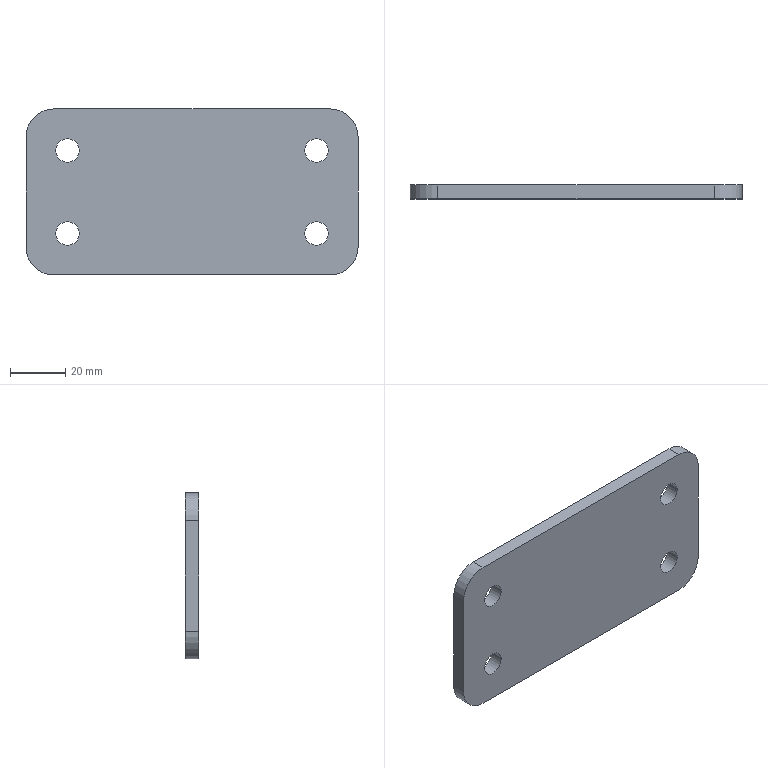Part | STEP file | JBJ-P-1007-05 | 1 solid | 14 faces | box 120 x 5 x 60 mm | volume 34436 mm3 | cylinder 8 | plane 6 | commonest cylinder face diameters 8.5 x4 20 x4
STEP:
#1=CARTESIAN_POINT('',(105.,5.,49.25));
#2=VERTEX_POINT('',#1);
#3=CARTESIAN_POINT('',(105.,5.,45.));
#4=DIRECTION('',(0.,1.,0.));
#5=DIRECTION('',(0.,0.,1.));
#6=AXIS2_PLACEMENT_3D('',#3,#4,#5);
#7=CIRCLE('',#6,4.25);
#8=EDGE_CURVE('',#2,#2,#7,.T.);
#9=ORIENTED_EDGE('',*,*,#8,.F.);
#10=EDGE_LOOP('',(#9));
#11=FACE_BOUND('',#10,.T.);
#12=CARTESIAN_POINT('',(15.,5.,19.25));
#13=VERTEX_POINT('',#12);
#14=CARTESIAN_POINT('',(15.,5.,15.));
#15=DIRECTION('',(0.,1.,0.));
#16=DIRECTION('',(0.,0.,1.));
#17=AXIS2_PLACEMENT_3D('',#14,#15,#16);
#18=CIRCLE('',#17,4.25);
#19=EDGE_CURVE('',#13,#13,#18,.T.);
#20=ORIENTED_EDGE('',*,*,#19,.F.);
#21=EDGE_LOOP('',(#20));
#22=FACE_BOUND('',#21,.T.);
#23=CARTESIAN_POINT('',(0.,5.,10.));
#24=VERTEX_POINT('',#23);
#25=CARTESIAN_POINT('',(0.,5.,50.));
#26=VERTEX_POINT('',#25);
#27=CARTESIAN_POINT('',(0.,5.,0.));
#28=DIRECTION('',(0.,0.,1.));
#29=VECTOR('',#28,1000.);
#30=LINE('',#27,#29);
#31=EDGE_CURVE('',#24,#26,#30,.T.);
#32=ORIENTED_EDGE('',*,*,#31,.T.);
#33=CARTESIAN_POINT('',(10.,5.,60.));
#34=VERTEX_POINT('',#33);
#35=CARTESIAN_POINT('',(10.,5.,50.));
#36=DIRECTION('',(0.,1.,0.));
#37=DIRECTION('',(0.,0.,1.));
#38=AXIS2_PLACEMENT_3D('',#35,#36,#37);
#39=CIRCLE('',#38,10.);
#40=EDGE_CURVE('',#26,#34,#39,.T.);
#41=ORIENTED_EDGE('',*,*,#40,.T.);
#42=CARTESIAN_POINT('',(110.,5.,60.));
#43=VERTEX_POINT('',#42);
#44=CARTESIAN_POINT('',(0.,5.,60.));
#45=DIRECTION('',(1.,0.,0.));
#46=VECTOR('',#45,1000.);
#47=LINE('',#44,#46);
#48=EDGE_CURVE('',#34,#43,#47,.T.);
#49=ORIENTED_EDGE('',*,*,#48,.T.);
#50=CARTESIAN_POINT('',(120.,5.,50.));
#51=VERTEX_POINT('',#50);
#52=CARTESIAN_POINT('',(110.,5.,50.));
#53=DIRECTION('',(0.,1.,0.));
#54=DIRECTION('',(0.,0.,1.));
#55=AXIS2_PLACEMENT_3D('',#52,#53,#54);
#56=CIRCLE('',#55,10.);
#57=EDGE_CURVE('',#43,#51,#56,.T.);
#58=ORIENTED_EDGE('',*,*,#57,.T.);
#59=CARTESIAN_POINT('',(120.,5.,10.));
#60=VERTEX_POINT('',#59);
#61=CARTESIAN_POINT('',(120.,5.,0.));
#62=DIRECTION('',(0.,0.,-1.));
#63=VECTOR('',#62,1000.);
#64=LINE('',#61,#63);
#65=EDGE_CURVE('',#51,#60,#64,.T.);
#66=ORIENTED_EDGE('',*,*,#65,.T.);
#67=CARTESIAN_POINT('',(110.,5.,0.));
#68=VERTEX_POINT('',#67);
#69=CARTESIAN_POINT('',(110.,5.,10.));
#70=DIRECTION('',(0.,1.,0.));
#71=DIRECTION('',(0.,0.,1.));
#72=AXIS2_PLACEMENT_3D('',#69,#70,#71);
#73=CIRCLE('',#72,10.);
#74=EDGE_CURVE('',#60,#68,#73,.T.);
#75=ORIENTED_EDGE('',*,*,#74,.T.);
#76=CARTESIAN_POINT('',(10.,5.,0.));
#77=VERTEX_POINT('',#76);
#78=CARTESIAN_POINT('',(0.,5.,0.));
#79=DIRECTION('',(-1.,0.,0.));
#80=VECTOR('',#79,1000.);
#81=LINE('',#78,#80);
#82=EDGE_CURVE('',#68,#77,#81,.T.);
#83=ORIENTED_EDGE('',*,*,#82,.T.);
#84=CARTESIAN_POINT('',(10.,5.,10.));
#85=DIRECTION('',(0.,1.,0.));
#86=DIRECTION('',(0.,0.,1.));
#87=AXIS2_PLACEMENT_3D('',#84,#85,#86);
#88=CIRCLE('',#87,10.);
#89=EDGE_CURVE('',#77,#24,#88,.T.);
#90=ORIENTED_EDGE('',*,*,#89,.T.);
#91=EDGE_LOOP('',(#32,#41,#49,#58,#66,#75,#83,#90));
#92=FACE_OUTER_BOUND('',#91,.T.);
#93=CARTESIAN_POINT('',(15.,5.,40.75));
#94=VERTEX_POINT('',#93);
#95=CARTESIAN_POINT('',(15.,5.,45.));
#96=DIRECTION('',(0.,1.,0.));
#97=DIRECTION('',(0.,0.,-1.));
#98=AXIS2_PLACEMENT_3D('',#95,#96,#97);
#99=CIRCLE('',#98,4.25);
#100=EDGE_CURVE('',#94,#94,#99,.T.);
#101=ORIENTED_EDGE('',*,*,#100,.F.);
#102=EDGE_LOOP('',(#101));
#103=FACE_BOUND('',#102,.T.);
#104=CARTESIAN_POINT('',(105.,5.,10.75));
#105=VERTEX_POINT('',#104);
#106=CARTESIAN_POINT('',(105.,5.,15.));
#107=DIRECTION('',(0.,1.,0.));
#108=DIRECTION('',(0.,0.,-1.));
#109=AXIS2_PLACEMENT_3D('',#106,#107,#108);
#110=CIRCLE('',#109,4.25);
#111=EDGE_CURVE('',#105,#105,#110,.T.);
#112=ORIENTED_EDGE('',*,*,#111,.F.);
#113=EDGE_LOOP('',(#112));
#114=FACE_BOUND('',#113,.T.);
#115=CARTESIAN_POINT('',(0.,5.,0.));
#116=DIRECTION('',(0.,1.,0.));
#117=DIRECTION('',(0.,0.,1.));
#118=AXIS2_PLACEMENT_3D('',#115,#116,#117);
#119=PLANE('',#118);
#120=ADVANCED_FACE('',(#11,#22,#92,#103,#114),#119,.T.);
#121=CARTESIAN_POINT('',(10.,0.,60.));
#122=VERTEX_POINT('',#121);
#123=CARTESIAN_POINT('',(110.,0.,60.));
#124=VERTEX_POINT('',#123);
#125=CARTESIAN_POINT('',(0.,0.,60.));
#126=DIRECTION('',(1.,0.,0.));
#127=VECTOR('',#126,1000.);
#128=LINE('',#125,#127);
#129=EDGE_CURVE('',#122,#124,#128,.T.);
#130=ORIENTED_EDGE('',*,*,#129,.F.);
#131=CARTESIAN_POINT('',(0.,0.,50.));
#132=VERTEX_POINT('',#131);
#133=CARTESIAN_POINT('',(10.,0.,50.));
#134=DIRECTION('',(0.,-1.,0.));
#135=DIRECTION('',(0.,0.,1.));
#136=AXIS2_PLACEMENT_3D('',#133,#134,#135);
#137=CIRCLE('',#136,10.);
#138=EDGE_CURVE('',#122,#132,#137,.T.);
#139=ORIENTED_EDGE('',*,*,#138,.T.);
#140=CARTESIAN_POINT('',(0.,0.,10.));
#141=VERTEX_POINT('',#140);
#142=CARTESIAN_POINT('',(0.,0.,0.));
#143=DIRECTION('',(0.,0.,1.));
#144=VECTOR('',#143,1000.);
#145=LINE('',#142,#144);
#146=EDGE_CURVE('',#141,#132,#145,.T.);
#147=ORIENTED_EDGE('',*,*,#146,.F.);
#148=CARTESIAN_POINT('',(10.,0.,0.));
#149=VERTEX_POINT('',#148);
#150=CARTESIAN_POINT('',(10.,0.,10.));
#151=DIRECTION('',(0.,-1.,0.));
#152=DIRECTION('',(0.,0.,1.));
#153=AXIS2_PLACEMENT_3D('',#150,#151,#152);
#154=CIRCLE('',#153,10.);
#155=EDGE_CURVE('',#141,#149,#154,.T.);
#156=ORIENTED_EDGE('',*,*,#155,.T.);
#157=CARTESIAN_POINT('',(110.,0.,0.));
#158=VERTEX_POINT('',#157);
#159=CARTESIAN_POINT('',(0.,0.,0.));
#160=DIRECTION('',(-1.,0.,0.));
#161=VECTOR('',#160,1000.);
#162=LINE('',#159,#161);
#163=EDGE_CURVE('',#158,#149,#162,.T.);
#164=ORIENTED_EDGE('',*,*,#163,.F.);
#165=CARTESIAN_POINT('',(120.,0.,10.));
#166=VERTEX_POINT('',#165);
#167=CARTESIAN_POINT('',(110.,0.,10.));
#168=DIRECTION('',(0.,-1.,0.));
#169=DIRECTION('',(0.,0.,1.));
#170=AXIS2_PLACEMENT_3D('',#167,#168,#169);
#171=CIRCLE('',#170,10.);
#172=EDGE_CURVE('',#158,#166,#171,.T.);
#173=ORIENTED_EDGE('',*,*,#172,.T.);
#174=CARTESIAN_POINT('',(120.,0.,50.));
#175=VERTEX_POINT('',#174);
#176=CARTESIAN_POINT('',(120.,0.,0.));
#177=DIRECTION('',(0.,0.,-1.));
#178=VECTOR('',#177,1000.);
#179=LINE('',#176,#178);
#180=EDGE_CURVE('',#175,#166,#179,.T.);
#181=ORIENTED_EDGE('',*,*,#180,.F.);
#182=CARTESIAN_POINT('',(110.,0.,50.));
#183=DIRECTION('',(0.,-1.,0.));
#184=DIRECTION('',(0.,0.,1.));
#185=AXIS2_PLACEMENT_3D('',#182,#183,#184);
#186=CIRCLE('',#185,10.);
#187=EDGE_CURVE('',#175,#124,#186,.T.);
#188=ORIENTED_EDGE('',*,*,#187,.T.);
#189=EDGE_LOOP('',(#130,#139,#147,#156,#164,#173,#181,#188));
#190=FACE_OUTER_BOUND('',#189,.T.);
#191=CARTESIAN_POINT('',(15.,0.,19.25));
#192=VERTEX_POINT('',#191);
#193=CARTESIAN_POINT('',(15.,0.,15.));
#194=DIRECTION('',(0.,1.,0.));
#195=DIRECTION('',(0.,0.,1.));
#196=AXIS2_PLACEMENT_3D('',#193,#194,#195);
#197=CIRCLE('',#196,4.25);
#198=EDGE_CURVE('',#192,#192,#197,.T.);
#199=ORIENTED_EDGE('',*,*,#198,.T.);
#200=EDGE_LOOP('',(#199));
#201=FACE_BOUND('',#200,.T.);
#202=CARTESIAN_POINT('',(15.,0.,40.75));
#203=VERTEX_POINT('',#202);
#204=CARTESIAN_POINT('',(15.,0.,45.));
#205=DIRECTION('',(0.,1.,0.));
#206=DIRECTION('',(0.,0.,-1.));
#207=AXIS2_PLACEMENT_3D('',#204,#205,#206);
#208=CIRCLE('',#207,4.25);
#209=EDGE_CURVE('',#203,#203,#208,.T.);
#210=ORIENTED_EDGE('',*,*,#209,.T.);
#211=EDGE_LOOP('',(#210));
#212=FACE_BOUND('',#211,.T.);
#213=CARTESIAN_POINT('',(105.,0.,49.25));
#214=VERTEX_POINT('',#213);
#215=CARTESIAN_POINT('',(105.,0.,45.));
#216=DIRECTION('',(0.,1.,0.));
#217=DIRECTION('',(0.,0.,1.));
#218=AXIS2_PLACEMENT_3D('',#215,#216,#217);
#219=CIRCLE('',#218,4.25);
#220=EDGE_CURVE('',#214,#214,#219,.T.);
#221=ORIENTED_EDGE('',*,*,#220,.T.);
#222=EDGE_LOOP('',(#221));
#223=FACE_BOUND('',#222,.T.);
#224=CARTESIAN_POINT('',(105.,0.,10.75));
#225=VERTEX_POINT('',#224);
#226=CARTESIAN_POINT('',(105.,0.,15.));
#227=DIRECTION('',(0.,1.,0.));
#228=DIRECTION('',(0.,0.,-1.));
#229=AXIS2_PLACEMENT_3D('',#226,#227,#228);
#230=CIRCLE('',#229,4.25);
#231=EDGE_CURVE('',#225,#225,#230,.T.);
#232=ORIENTED_EDGE('',*,*,#231,.T.);
#233=EDGE_LOOP('',(#232));
#234=FACE_BOUND('',#233,.T.);
#235=CARTESIAN_POINT('',(0.,0.,0.));
#236=DIRECTION('',(0.,1.,0.));
#237=DIRECTION('',(0.,0.,1.));
#238=AXIS2_PLACEMENT_3D('',#235,#236,#237);
#239=PLANE('',#238);
#240=ADVANCED_FACE('',(#190,#201,#212,#223,#234),#239,.F.);
#241=ORIENTED_EDGE('',*,*,#146,.T.);
#242=CARTESIAN_POINT('',(0.,5.,50.));
#243=DIRECTION('',(0.,1.,0.));
#244=VECTOR('',#243,1000.);
#245=LINE('',#242,#244);
#246=EDGE_CURVE('',#132,#26,#245,.T.);
#247=ORIENTED_EDGE('',*,*,#246,.T.);
#248=ORIENTED_EDGE('',*,*,#31,.F.);
#249=CARTESIAN_POINT('',(0.,5.,10.));
#250=DIRECTION('',(0.,-1.,0.));
#251=VECTOR('',#250,1000.);
#252=LINE('',#249,#251);
#253=EDGE_CURVE('',#24,#141,#252,.T.);
#254=ORIENTED_EDGE('',*,*,#253,.T.);
#255=EDGE_LOOP('',(#241,#247,#248,#254));
#256=FACE_OUTER_BOUND('',#255,.T.);
#257=CARTESIAN_POINT('',(0.,5.,0.));
#258=DIRECTION('',(1.,0.,0.));
#259=DIRECTION('',(0.,0.,-1.));
#260=AXIS2_PLACEMENT_3D('',#257,#258,#259);
#261=PLANE('',#260);
#262=ADVANCED_FACE('',(#256),#261,.F.);
#263=ORIENTED_EDGE('',*,*,#48,.F.);
#264=CARTESIAN_POINT('',(10.,5.,60.));
#265=DIRECTION('',(0.,-1.,0.));
#266=VECTOR('',#265,1000.);
#267=LINE('',#264,#266);
#268=EDGE_CURVE('',#34,#122,#267,.T.);
#269=ORIENTED_EDGE('',*,*,#268,.T.);
#270=ORIENTED_EDGE('',*,*,#129,.T.);
#271=CARTESIAN_POINT('',(110.,5.,60.));
#272=DIRECTION('',(0.,1.,0.));
#273=VECTOR('',#272,1000.);
#274=LINE('',#271,#273);
#275=EDGE_CURVE('',#124,#43,#274,.T.);
#276=ORIENTED_EDGE('',*,*,#275,.T.);
#277=EDGE_LOOP('',(#263,#269,#270,#276));
#278=FACE_OUTER_BOUND('',#277,.T.);
#279=CARTESIAN_POINT('',(0.,5.,60.));
#280=DIRECTION('',(0.,0.,-1.));
#281=DIRECTION('',(-1.,0.,0.));
#282=AXIS2_PLACEMENT_3D('',#279,#280,#281);
#283=PLANE('',#282);
#284=ADVANCED_FACE('',(#278),#283,.F.);
#285=ORIENTED_EDGE('',*,*,#180,.T.);
#286=CARTESIAN_POINT('',(120.,5.,10.));
#287=DIRECTION('',(0.,1.,0.));
#288=VECTOR('',#287,1000.);
#289=LINE('',#286,#288);
#290=EDGE_CURVE('',#166,#60,#289,.T.);
#291=ORIENTED_EDGE('',*,*,#290,.T.);
#292=ORIENTED_EDGE('',*,*,#65,.F.);
#293=CARTESIAN_POINT('',(120.,5.,50.));
#294=DIRECTION('',(0.,-1.,0.));
#295=VECTOR('',#294,1000.);
#296=LINE('',#293,#295);
#297=EDGE_CURVE('',#51,#175,#296,.T.);
#298=ORIENTED_EDGE('',*,*,#297,.T.);
#299=EDGE_LOOP('',(#285,#291,#292,#298));
#300=FACE_OUTER_BOUND('',#299,.T.);
#301=CARTESIAN_POINT('',(120.,5.,0.));
#302=DIRECTION('',(-1.,0.,0.));
#303=DIRECTION('',(0.,0.,1.));
#304=AXIS2_PLACEMENT_3D('',#301,#302,#303);
#305=PLANE('',#304);
#306=ADVANCED_FACE('',(#300),#305,.F.);
#307=ORIENTED_EDGE('',*,*,#163,.T.);
#308=CARTESIAN_POINT('',(10.,5.,0.));
#309=DIRECTION('',(0.,1.,0.));
#310=VECTOR('',#309,1000.);
#311=LINE('',#308,#310);
#312=EDGE_CURVE('',#149,#77,#311,.T.);
#313=ORIENTED_EDGE('',*,*,#312,.T.);
#314=ORIENTED_EDGE('',*,*,#82,.F.);
#315=CARTESIAN_POINT('',(110.,5.,0.));
#316=DIRECTION('',(0.,-1.,0.));
#317=VECTOR('',#316,1000.);
#318=LINE('',#315,#317);
#319=EDGE_CURVE('',#68,#158,#318,.T.);
#320=ORIENTED_EDGE('',*,*,#319,.T.);
#321=EDGE_LOOP('',(#307,#313,#314,#320));
#322=FACE_OUTER_BOUND('',#321,.T.);
#323=CARTESIAN_POINT('',(0.,5.,0.));
#324=DIRECTION('',(0.,0.,1.));
#325=DIRECTION('',(1.,0.,0.));
#326=AXIS2_PLACEMENT_3D('',#323,#324,#325);
#327=PLANE('',#326);
#328=ADVANCED_FACE('',(#322),#327,.F.);
#329=ORIENTED_EDGE('',*,*,#19,.T.);
#330=EDGE_LOOP('',(#329));
#331=FACE_OUTER_BOUND('',#330,.T.);
#332=ORIENTED_EDGE('',*,*,#198,.F.);
#333=EDGE_LOOP('',(#332));
#334=FACE_OUTER_BOUND('',#333,.T.);
#335=CARTESIAN_POINT('',(15.,5.,15.));
#336=DIRECTION('',(0.,-1.,0.));
#337=DIRECTION('',(0.,0.,-1.));
#338=AXIS2_PLACEMENT_3D('',#335,#336,#337);
#339=CYLINDRICAL_SURFACE('',#338,4.25);
#340=ADVANCED_FACE('',(#331,#334),#339,.F.);
#341=ORIENTED_EDGE('',*,*,#100,.T.);
#342=EDGE_LOOP('',(#341));
#343=FACE_OUTER_BOUND('',#342,.T.);
#344=ORIENTED_EDGE('',*,*,#209,.F.);
#345=EDGE_LOOP('',(#344));
#346=FACE_OUTER_BOUND('',#345,.T.);
#347=CARTESIAN_POINT('',(15.,5.,45.));
#348=DIRECTION('',(0.,-1.,0.));
#349=DIRECTION('',(0.,0.,-1.));
#350=AXIS2_PLACEMENT_3D('',#347,#348,#349);
#351=CYLINDRICAL_SURFACE('',#350,4.25);
#352=ADVANCED_FACE('',(#343,#346),#351,.F.);
#353=ORIENTED_EDGE('',*,*,#8,.T.);
#354=EDGE_LOOP('',(#353));
#355=FACE_OUTER_BOUND('',#354,.T.);
#356=ORIENTED_EDGE('',*,*,#220,.F.);
#357=EDGE_LOOP('',(#356));
#358=FACE_OUTER_BOUND('',#357,.T.);
#359=CARTESIAN_POINT('',(105.,5.,45.));
#360=DIRECTION('',(0.,-1.,0.));
#361=DIRECTION('',(0.,0.,-1.));
#362=AXIS2_PLACEMENT_3D('',#359,#360,#361);
#363=CYLINDRICAL_SURFACE('',#362,4.25);
#364=ADVANCED_FACE('',(#355,#358),#363,.F.);
#365=ORIENTED_EDGE('',*,*,#111,.T.);
#366=EDGE_LOOP('',(#365));
#367=FACE_OUTER_BOUND('',#366,.T.);
#368=ORIENTED_EDGE('',*,*,#231,.F.);
#369=EDGE_LOOP('',(#368));
#370=FACE_OUTER_BOUND('',#369,.T.);
#371=CARTESIAN_POINT('',(105.,5.,15.));
#372=DIRECTION('',(0.,-1.,0.));
#373=DIRECTION('',(0.,0.,-1.));
#374=AXIS2_PLACEMENT_3D('',#371,#372,#373);
#375=CYLINDRICAL_SURFACE('',#374,4.25);
#376=ADVANCED_FACE('',(#367,#370),#375,.F.);
#377=ORIENTED_EDGE('',*,*,#40,.F.);
#378=ORIENTED_EDGE('',*,*,#246,.F.);
#379=ORIENTED_EDGE('',*,*,#138,.F.);
#380=ORIENTED_EDGE('',*,*,#268,.F.);
#381=EDGE_LOOP('',(#377,#378,#379,#380));
#382=FACE_OUTER_BOUND('',#381,.T.);
#383=CARTESIAN_POINT('',(10.,5.,50.));
#384=DIRECTION('',(0.,-1.,0.));
#385=DIRECTION('',(0.,0.,-1.));
#386=AXIS2_PLACEMENT_3D('',#383,#384,#385);
#387=CYLINDRICAL_SURFACE('',#386,10.);
#388=ADVANCED_FACE('',(#382),#387,.T.);
#389=ORIENTED_EDGE('',*,*,#89,.F.);
#390=ORIENTED_EDGE('',*,*,#312,.F.);
#391=ORIENTED_EDGE('',*,*,#155,.F.);
#392=ORIENTED_EDGE('',*,*,#253,.F.);
#393=EDGE_LOOP('',(#389,#390,#391,#392));
#394=FACE_OUTER_BOUND('',#393,.T.);
#395=CARTESIAN_POINT('',(10.,5.,10.));
#396=DIRECTION('',(0.,-1.,0.));
#397=DIRECTION('',(0.,0.,-1.));
#398=AXIS2_PLACEMENT_3D('',#395,#396,#397);
#399=CYLINDRICAL_SURFACE('',#398,10.);
#400=ADVANCED_FACE('',(#394),#399,.T.);
#401=ORIENTED_EDGE('',*,*,#74,.F.);
#402=ORIENTED_EDGE('',*,*,#290,.F.);
#403=ORIENTED_EDGE('',*,*,#172,.F.);
#404=ORIENTED_EDGE('',*,*,#319,.F.);
#405=EDGE_LOOP('',(#401,#402,#403,#404));
#406=FACE_OUTER_BOUND('',#405,.T.);
#407=CARTESIAN_POINT('',(110.,5.,10.));
#408=DIRECTION('',(0.,-1.,0.));
#409=DIRECTION('',(0.,0.,-1.));
#410=AXIS2_PLACEMENT_3D('',#407,#408,#409);
#411=CYLINDRICAL_SURFACE('',#410,10.);
#412=ADVANCED_FACE('',(#406),#411,.T.);
#413=ORIENTED_EDGE('',*,*,#57,.F.);
#414=ORIENTED_EDGE('',*,*,#275,.F.);
#415=ORIENTED_EDGE('',*,*,#187,.F.);
#416=ORIENTED_EDGE('',*,*,#297,.F.);
#417=EDGE_LOOP('',(#413,#414,#415,#416));
#418=FACE_OUTER_BOUND('',#417,.T.);
#419=CARTESIAN_POINT('',(110.,5.,50.));
#420=DIRECTION('',(0.,-1.,0.));
#421=DIRECTION('',(0.,0.,-1.));
#422=AXIS2_PLACEMENT_3D('',#419,#420,#421);
#423=CYLINDRICAL_SURFACE('',#422,10.);
#424=ADVANCED_FACE('',(#418),#423,.T.);
#425=CLOSED_SHELL('',(#120,#240,#262,#284,#306,#328,#340,#352,#364,#376,#388,#400,#412,#424));
#426=MANIFOLD_SOLID_BREP('',#425);
#427=CARTESIAN_POINT('',(0.,0.,0.));
#428=DIRECTION('',(0.,0.,1.));
#429=DIRECTION('',(1.,0.,0.));
#430=AXIS2_PLACEMENT_3D('',#427,#428,#429);
#431=(LENGTH_UNIT()NAMED_UNIT(*)SI_UNIT(.MILLI.,.METRE.));
#432=UNCERTAINTY_MEASURE_WITH_UNIT(LENGTH_MEASURE(0.00001),#431,'','');
#433=(NAMED_UNIT(*)PLANE_ANGLE_UNIT()SI_UNIT($,.RADIAN.));
#434=(NAMED_UNIT(*)SI_UNIT($,.STERADIAN.)SOLID_ANGLE_UNIT());
#435=(GEOMETRIC_REPRESENTATION_CONTEXT(3)GLOBAL_UNCERTAINTY_ASSIGNED_CONTEXT((#432))GLOBAL_UNIT_ASSIGNED_CONTEXT((#431,#433,#434))REPRESENTATION_CONTEXT('',''));
#436=ADVANCED_BREP_SHAPE_REPRESENTATION('',(#426,#430),#435);